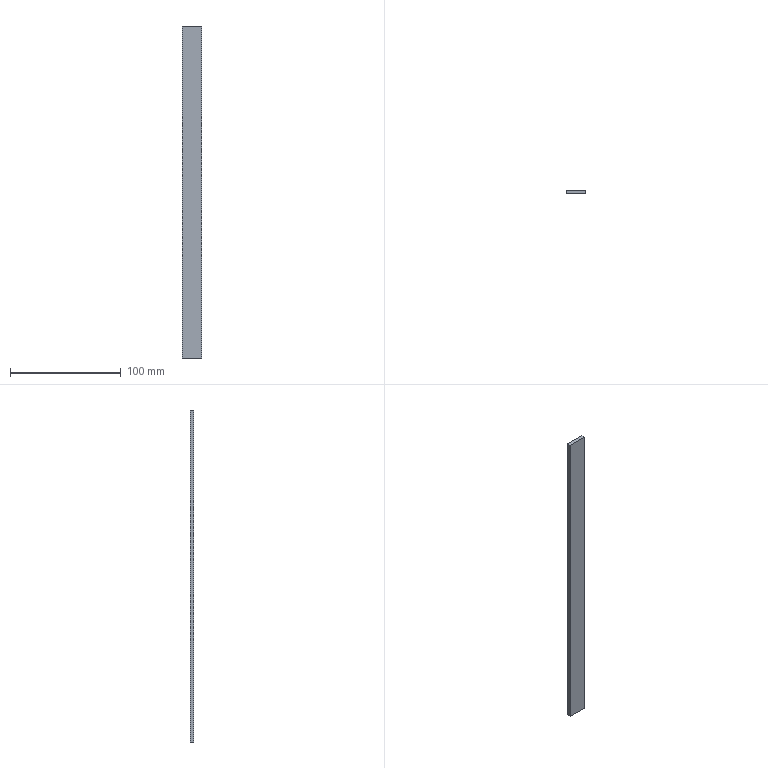Part | SolidWorks | features Extrusion 1 | 1 solid | 6 faces | box 18 x 3 x 300 mm | volume 16200 mm3 | plane 6
STEP:
#1=CARTESIAN_POINT('',(9.,-1.5,0.));
#2=VERTEX_POINT('',#1);
#3=CARTESIAN_POINT('',(9.,1.5,0.));
#4=VERTEX_POINT('',#3);
#5=CARTESIAN_POINT('',(9.,1.5,0.));
#6=DIRECTION('',(0.,1.,0.));
#7=VECTOR('',#6,1000.);
#8=LINE('',#5,#7);
#9=EDGE_CURVE('',#2,#4,#8,.T.);
#10=ORIENTED_EDGE('',*,*,#9,.T.);
#11=CARTESIAN_POINT('',(9.,1.5,300.));
#12=VERTEX_POINT('',#11);
#13=CARTESIAN_POINT('',(9.,1.5,300.));
#14=DIRECTION('',(0.,0.,-1.));
#15=VECTOR('',#14,1000.);
#16=LINE('',#13,#15);
#17=EDGE_CURVE('',#12,#4,#16,.T.);
#18=ORIENTED_EDGE('',*,*,#17,.F.);
#19=CARTESIAN_POINT('',(9.,-1.5,300.));
#20=VERTEX_POINT('',#19);
#21=CARTESIAN_POINT('',(9.,1.5,300.));
#22=DIRECTION('',(0.,1.,0.));
#23=VECTOR('',#22,1000.);
#24=LINE('',#21,#23);
#25=EDGE_CURVE('',#20,#12,#24,.T.);
#26=ORIENTED_EDGE('',*,*,#25,.F.);
#27=CARTESIAN_POINT('',(9.,-1.5,300.));
#28=DIRECTION('',(0.,0.,-1.));
#29=VECTOR('',#28,1000.);
#30=LINE('',#27,#29);
#31=EDGE_CURVE('',#20,#2,#30,.T.);
#32=ORIENTED_EDGE('',*,*,#31,.T.);
#33=EDGE_LOOP('',(#10,#18,#26,#32));
#34=FACE_OUTER_BOUND('',#33,.T.);
#35=CARTESIAN_POINT('',(9.,1.5,300.));
#36=DIRECTION('',(-1.,0.,0.));
#37=DIRECTION('',(0.,0.,1.));
#38=AXIS2_PLACEMENT_3D('',#35,#36,#37);
#39=PLANE('',#38);
#40=ADVANCED_FACE('',(#34),#39,.F.);
#41=CARTESIAN_POINT('',(-9.,1.5,0.));
#42=VERTEX_POINT('',#41);
#43=CARTESIAN_POINT('',(-9.,1.5,0.));
#44=DIRECTION('',(-1.,0.,0.));
#45=VECTOR('',#44,1000.);
#46=LINE('',#43,#45);
#47=EDGE_CURVE('',#4,#42,#46,.T.);
#48=ORIENTED_EDGE('',*,*,#47,.T.);
#49=CARTESIAN_POINT('',(-9.,1.5,300.));
#50=VERTEX_POINT('',#49);
#51=CARTESIAN_POINT('',(-9.,1.5,300.));
#52=DIRECTION('',(0.,0.,-1.));
#53=VECTOR('',#52,1000.);
#54=LINE('',#51,#53);
#55=EDGE_CURVE('',#50,#42,#54,.T.);
#56=ORIENTED_EDGE('',*,*,#55,.F.);
#57=CARTESIAN_POINT('',(-9.,1.5,300.));
#58=DIRECTION('',(-1.,0.,0.));
#59=VECTOR('',#58,1000.);
#60=LINE('',#57,#59);
#61=EDGE_CURVE('',#12,#50,#60,.T.);
#62=ORIENTED_EDGE('',*,*,#61,.F.);
#63=ORIENTED_EDGE('',*,*,#17,.T.);
#64=EDGE_LOOP('',(#48,#56,#62,#63));
#65=FACE_OUTER_BOUND('',#64,.T.);
#66=CARTESIAN_POINT('',(-9.,1.5,300.));
#67=DIRECTION('',(0.,-1.,0.));
#68=DIRECTION('',(0.,0.,-1.));
#69=AXIS2_PLACEMENT_3D('',#66,#67,#68);
#70=PLANE('',#69);
#71=ADVANCED_FACE('',(#65),#70,.F.);
#72=CARTESIAN_POINT('',(-9.,-1.5,0.));
#73=VERTEX_POINT('',#72);
#74=CARTESIAN_POINT('',(-9.,1.5,0.));
#75=DIRECTION('',(0.,-1.,0.));
#76=VECTOR('',#75,1000.);
#77=LINE('',#74,#76);
#78=EDGE_CURVE('',#42,#73,#77,.T.);
#79=ORIENTED_EDGE('',*,*,#78,.T.);
#80=CARTESIAN_POINT('',(-9.,-1.5,300.));
#81=VERTEX_POINT('',#80);
#82=CARTESIAN_POINT('',(-9.,-1.5,300.));
#83=DIRECTION('',(0.,0.,-1.));
#84=VECTOR('',#83,1000.);
#85=LINE('',#82,#84);
#86=EDGE_CURVE('',#81,#73,#85,.T.);
#87=ORIENTED_EDGE('',*,*,#86,.F.);
#88=CARTESIAN_POINT('',(-9.,1.5,300.));
#89=DIRECTION('',(0.,-1.,0.));
#90=VECTOR('',#89,1000.);
#91=LINE('',#88,#90);
#92=EDGE_CURVE('',#50,#81,#91,.T.);
#93=ORIENTED_EDGE('',*,*,#92,.F.);
#94=ORIENTED_EDGE('',*,*,#55,.T.);
#95=EDGE_LOOP('',(#79,#87,#93,#94));
#96=FACE_OUTER_BOUND('',#95,.T.);
#97=CARTESIAN_POINT('',(-9.,1.5,300.));
#98=DIRECTION('',(1.,0.,0.));
#99=DIRECTION('',(0.,0.,-1.));
#100=AXIS2_PLACEMENT_3D('',#97,#98,#99);
#101=PLANE('',#100);
#102=ADVANCED_FACE('',(#96),#101,.F.);
#103=CARTESIAN_POINT('',(-9.,-1.5,0.));
#104=DIRECTION('',(1.,0.,0.));
#105=VECTOR('',#104,1000.);
#106=LINE('',#103,#105);
#107=EDGE_CURVE('',#73,#2,#106,.T.);
#108=ORIENTED_EDGE('',*,*,#107,.T.);
#109=ORIENTED_EDGE('',*,*,#31,.F.);
#110=CARTESIAN_POINT('',(-9.,-1.5,300.));
#111=DIRECTION('',(1.,0.,0.));
#112=VECTOR('',#111,1000.);
#113=LINE('',#110,#112);
#114=EDGE_CURVE('',#81,#20,#113,.T.);
#115=ORIENTED_EDGE('',*,*,#114,.F.);
#116=ORIENTED_EDGE('',*,*,#86,.T.);
#117=EDGE_LOOP('',(#108,#109,#115,#116));
#118=FACE_OUTER_BOUND('',#117,.T.);
#119=CARTESIAN_POINT('',(-9.,-1.5,300.));
#120=DIRECTION('',(0.,1.,0.));
#121=DIRECTION('',(0.,0.,1.));
#122=AXIS2_PLACEMENT_3D('',#119,#120,#121);
#123=PLANE('',#122);
#124=ADVANCED_FACE('',(#118),#123,.F.);
#125=ORIENTED_EDGE('',*,*,#25,.T.);
#126=ORIENTED_EDGE('',*,*,#61,.T.);
#127=ORIENTED_EDGE('',*,*,#92,.T.);
#128=ORIENTED_EDGE('',*,*,#114,.T.);
#129=EDGE_LOOP('',(#125,#126,#127,#128));
#130=FACE_OUTER_BOUND('',#129,.T.);
#131=CARTESIAN_POINT('',(0.,0.,300.));
#132=DIRECTION('',(0.,0.,1.));
#133=DIRECTION('',(1.,0.,0.));
#134=AXIS2_PLACEMENT_3D('',#131,#132,#133);
#135=PLANE('',#134);
#136=ADVANCED_FACE('',(#130),#135,.T.);
#137=ORIENTED_EDGE('',*,*,#9,.F.);
#138=ORIENTED_EDGE('',*,*,#107,.F.);
#139=ORIENTED_EDGE('',*,*,#78,.F.);
#140=ORIENTED_EDGE('',*,*,#47,.F.);
#141=EDGE_LOOP('',(#137,#138,#139,#140));
#142=FACE_OUTER_BOUND('',#141,.T.);
#143=CARTESIAN_POINT('',(0.,0.,0.));
#144=DIRECTION('',(0.,0.,1.));
#145=DIRECTION('',(1.,0.,0.));
#146=AXIS2_PLACEMENT_3D('',#143,#144,#145);
#147=PLANE('',#146);
#148=ADVANCED_FACE('',(#142),#147,.F.);
#149=CLOSED_SHELL('',(#40,#71,#102,#124,#136,#148));
#150=MANIFOLD_SOLID_BREP('',#149);
#151=CARTESIAN_POINT('',(0.,0.,0.));
#152=DIRECTION('',(0.,0.,1.));
#153=DIRECTION('',(1.,0.,0.));
#154=AXIS2_PLACEMENT_3D('',#151,#152,#153);
#155=(LENGTH_UNIT()NAMED_UNIT(*)SI_UNIT(.MILLI.,.METRE.));
#156=UNCERTAINTY_MEASURE_WITH_UNIT(LENGTH_MEASURE(0.00001),#155,'','');
#157=(NAMED_UNIT(*)PLANE_ANGLE_UNIT()SI_UNIT($,.RADIAN.));
#158=(NAMED_UNIT(*)SI_UNIT($,.STERADIAN.)SOLID_ANGLE_UNIT());
#159=(GEOMETRIC_REPRESENTATION_CONTEXT(3)GLOBAL_UNCERTAINTY_ASSIGNED_CONTEXT((#156))GLOBAL_UNIT_ASSIGNED_CONTEXT((#155,#157,#158))REPRESENTATION_CONTEXT('',''));
#160=ADVANCED_BREP_SHAPE_REPRESENTATION('',(#150,#154),#159);